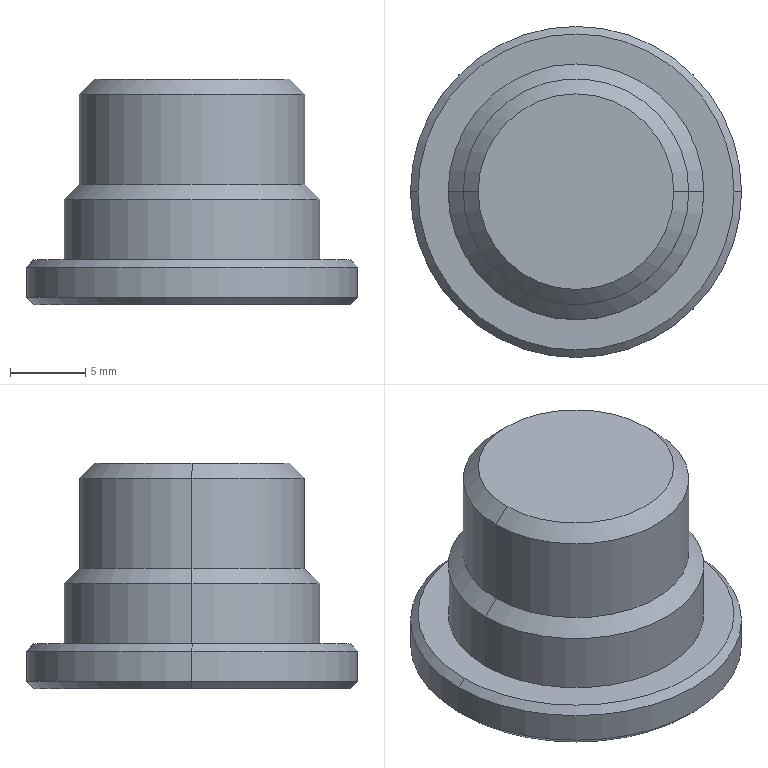Part | SolidWorks | features Chamfer 2, Revolution 1 | 1 solid | 17 faces | box 22 x 22 x 15 mm | volume 3447 mm3 | cone 8 | cylinder 6 | plane 3 | commonest cylinder face diameters 15 x2 17 x2 22 x2
STEP:
#1=CARTESIAN_POINT('',(10.5,0.,-12.));
#2=VERTEX_POINT('',#1);
#3=CARTESIAN_POINT('',(-10.5,0.,-12.));
#4=VERTEX_POINT('',#3);
#5=CARTESIAN_POINT('',(0.,0.,-12.));
#6=DIRECTION('',(0.,0.,1.));
#7=DIRECTION('',(-1.,0.,0.));
#8=AXIS2_PLACEMENT_3D('',#5,#6,#7);
#9=CIRCLE('',#8,10.5);
#10=EDGE_CURVE('',#2,#4,#9,.T.);
#11=ORIENTED_EDGE('',*,*,#10,.F.);
#12=CARTESIAN_POINT('',(11.,0.,-12.5));
#13=VERTEX_POINT('',#12);
#14=CARTESIAN_POINT('',(10.5,0.,-12.));
#15=DIRECTION('',(0.7071,0.,-0.7071));
#16=VECTOR('',#15,1000.);
#17=LINE('',#14,#16);
#18=EDGE_CURVE('',#2,#13,#17,.T.);
#19=ORIENTED_EDGE('',*,*,#18,.T.);
#20=CARTESIAN_POINT('',(-11.,0.,-12.5));
#21=VERTEX_POINT('',#20);
#22=CARTESIAN_POINT('',(0.,0.,-12.5));
#23=DIRECTION('',(0.,0.,-1.));
#24=DIRECTION('',(-1.,0.,0.));
#25=AXIS2_PLACEMENT_3D('',#22,#23,#24);
#26=CIRCLE('',#25,11.);
#27=EDGE_CURVE('',#21,#13,#26,.T.);
#28=ORIENTED_EDGE('',*,*,#27,.F.);
#29=CARTESIAN_POINT('',(-10.5,0.,-12.));
#30=DIRECTION('',(-0.7071,0.,-0.7071));
#31=VECTOR('',#30,1000.);
#32=LINE('',#29,#31);
#33=EDGE_CURVE('',#4,#21,#32,.T.);
#34=ORIENTED_EDGE('',*,*,#33,.F.);
#35=EDGE_LOOP('',(#11,#19,#28,#34));
#36=FACE_OUTER_BOUND('',#35,.T.);
#37=CARTESIAN_POINT('',(0.,0.,-12.));
#38=DIRECTION('',(0.,0.,-1.));
#39=DIRECTION('',(-1.,0.,0.));
#40=AXIS2_PLACEMENT_3D('',#37,#38,#39);
#41=CONICAL_SURFACE('',#40,10.5,0.7854);
#42=ADVANCED_FACE('',(#36),#41,.T.);
#43=CARTESIAN_POINT('',(-10.5,0.,-15.));
#44=VERTEX_POINT('',#43);
#45=CARTESIAN_POINT('',(10.5,0.,-15.));
#46=VERTEX_POINT('',#45);
#47=CARTESIAN_POINT('',(0.,0.,-15.));
#48=DIRECTION('',(0.,0.,-1.));
#49=DIRECTION('',(1.,0.,0.));
#50=AXIS2_PLACEMENT_3D('',#47,#48,#49);
#51=CIRCLE('',#50,10.5);
#52=EDGE_CURVE('',#44,#46,#51,.T.);
#53=ORIENTED_EDGE('',*,*,#52,.F.);
#54=CARTESIAN_POINT('',(-11.,0.,-14.5));
#55=VERTEX_POINT('',#54);
#56=CARTESIAN_POINT('',(-11.,0.,-14.5));
#57=DIRECTION('',(-0.7071,0.,0.7071));
#58=VECTOR('',#57,1000.);
#59=LINE('',#56,#58);
#60=EDGE_CURVE('',#44,#55,#59,.T.);
#61=ORIENTED_EDGE('',*,*,#60,.T.);
#62=CARTESIAN_POINT('',(11.,0.,-14.5));
#63=VERTEX_POINT('',#62);
#64=CARTESIAN_POINT('',(0.,0.,-14.5));
#65=DIRECTION('',(0.,0.,1.));
#66=DIRECTION('',(1.,0.,0.));
#67=AXIS2_PLACEMENT_3D('',#64,#65,#66);
#68=CIRCLE('',#67,11.);
#69=EDGE_CURVE('',#63,#55,#68,.T.);
#70=ORIENTED_EDGE('',*,*,#69,.F.);
#71=CARTESIAN_POINT('',(11.,0.,-14.5));
#72=DIRECTION('',(0.7071,0.,0.7071));
#73=VECTOR('',#72,1000.);
#74=LINE('',#71,#73);
#75=EDGE_CURVE('',#46,#63,#74,.T.);
#76=ORIENTED_EDGE('',*,*,#75,.F.);
#77=EDGE_LOOP('',(#53,#61,#70,#76));
#78=FACE_OUTER_BOUND('',#77,.T.);
#79=CARTESIAN_POINT('',(0.,0.,-14.5));
#80=DIRECTION('',(0.,0.,1.));
#81=DIRECTION('',(1.,0.,0.));
#82=AXIS2_PLACEMENT_3D('',#79,#80,#81);
#83=CONICAL_SURFACE('',#82,11.,0.7854);
#84=ADVANCED_FACE('',(#78),#83,.T.);
#85=CARTESIAN_POINT('',(6.5,0.,0.));
#86=VERTEX_POINT('',#85);
#87=CARTESIAN_POINT('',(-6.5,0.,0.));
#88=VERTEX_POINT('',#87);
#89=CARTESIAN_POINT('',(0.,0.,0.));
#90=DIRECTION('',(0.,0.,1.));
#91=DIRECTION('',(-1.,0.,0.));
#92=AXIS2_PLACEMENT_3D('',#89,#90,#91);
#93=CIRCLE('',#92,6.5);
#94=EDGE_CURVE('',#86,#88,#93,.T.);
#95=ORIENTED_EDGE('',*,*,#94,.F.);
#96=CARTESIAN_POINT('',(7.5,0.,-1.));
#97=VERTEX_POINT('',#96);
#98=CARTESIAN_POINT('',(6.5,0.,0.));
#99=DIRECTION('',(0.7071,0.,-0.7071));
#100=VECTOR('',#99,1000.);
#101=LINE('',#98,#100);
#102=EDGE_CURVE('',#86,#97,#101,.T.);
#103=ORIENTED_EDGE('',*,*,#102,.T.);
#104=CARTESIAN_POINT('',(-7.5,0.,-1.));
#105=VERTEX_POINT('',#104);
#106=CARTESIAN_POINT('',(0.,0.,-1.));
#107=DIRECTION('',(0.,0.,-1.));
#108=DIRECTION('',(-1.,0.,0.));
#109=AXIS2_PLACEMENT_3D('',#106,#107,#108);
#110=CIRCLE('',#109,7.5);
#111=EDGE_CURVE('',#105,#97,#110,.T.);
#112=ORIENTED_EDGE('',*,*,#111,.F.);
#113=CARTESIAN_POINT('',(-6.5,0.,0.));
#114=DIRECTION('',(-0.7071,0.,-0.7071));
#115=VECTOR('',#114,1000.);
#116=LINE('',#113,#115);
#117=EDGE_CURVE('',#88,#105,#116,.T.);
#118=ORIENTED_EDGE('',*,*,#117,.F.);
#119=EDGE_LOOP('',(#95,#103,#112,#118));
#120=FACE_OUTER_BOUND('',#119,.T.);
#121=CARTESIAN_POINT('',(0.,0.,0.));
#122=DIRECTION('',(0.,0.,-1.));
#123=DIRECTION('',(-1.,0.,0.));
#124=AXIS2_PLACEMENT_3D('',#121,#122,#123);
#125=CONICAL_SURFACE('',#124,6.5,0.7854);
#126=ADVANCED_FACE('',(#120),#125,.T.);
#127=CARTESIAN_POINT('',(7.5,0.,-7.));
#128=VERTEX_POINT('',#127);
#129=CARTESIAN_POINT('',(-7.5,0.,-7.));
#130=VERTEX_POINT('',#129);
#131=CARTESIAN_POINT('',(0.,0.,-7.));
#132=DIRECTION('',(0.,0.,1.));
#133=DIRECTION('',(1.,0.,0.));
#134=AXIS2_PLACEMENT_3D('',#131,#132,#133);
#135=CIRCLE('',#134,7.5);
#136=EDGE_CURVE('',#128,#130,#135,.T.);
#137=ORIENTED_EDGE('',*,*,#136,.F.);
#138=CARTESIAN_POINT('',(8.5,0.,-8.));
#139=VERTEX_POINT('',#138);
#140=CARTESIAN_POINT('',(7.5,0.,-7.));
#141=DIRECTION('',(0.7071,0.,-0.7071));
#142=VECTOR('',#141,1000.);
#143=LINE('',#140,#142);
#144=EDGE_CURVE('',#128,#139,#143,.T.);
#145=ORIENTED_EDGE('',*,*,#144,.T.);
#146=CARTESIAN_POINT('',(-8.5,0.,-8.));
#147=VERTEX_POINT('',#146);
#148=CARTESIAN_POINT('',(0.,0.,-8.));
#149=DIRECTION('',(0.,0.,-1.));
#150=DIRECTION('',(-1.,0.,0.));
#151=AXIS2_PLACEMENT_3D('',#148,#149,#150);
#152=CIRCLE('',#151,8.5);
#153=EDGE_CURVE('',#147,#139,#152,.T.);
#154=ORIENTED_EDGE('',*,*,#153,.F.);
#155=CARTESIAN_POINT('',(-7.5,0.,-7.));
#156=DIRECTION('',(-0.7071,0.,-0.7071));
#157=VECTOR('',#156,1000.);
#158=LINE('',#155,#157);
#159=EDGE_CURVE('',#130,#147,#158,.T.);
#160=ORIENTED_EDGE('',*,*,#159,.F.);
#161=EDGE_LOOP('',(#137,#145,#154,#160));
#162=FACE_OUTER_BOUND('',#161,.T.);
#163=CARTESIAN_POINT('',(0.,0.,-7.));
#164=DIRECTION('',(0.,0.,-1.));
#165=DIRECTION('',(-1.,0.,0.));
#166=AXIS2_PLACEMENT_3D('',#163,#164,#165);
#167=CONICAL_SURFACE('',#166,7.5,0.7854);
#168=ADVANCED_FACE('',(#162),#167,.T.);
#169=ORIENTED_EDGE('',*,*,#69,.T.);
#170=CARTESIAN_POINT('',(-11.,0.,0.));
#171=DIRECTION('',(0.,0.,1.));
#172=VECTOR('',#171,1000.);
#173=LINE('',#170,#172);
#174=EDGE_CURVE('',#55,#21,#173,.T.);
#175=ORIENTED_EDGE('',*,*,#174,.T.);
#176=ORIENTED_EDGE('',*,*,#27,.T.);
#177=CARTESIAN_POINT('',(11.,0.,0.));
#178=DIRECTION('',(0.,0.,1.));
#179=VECTOR('',#178,1000.);
#180=LINE('',#177,#179);
#181=EDGE_CURVE('',#63,#13,#180,.T.);
#182=ORIENTED_EDGE('',*,*,#181,.F.);
#183=EDGE_LOOP('',(#169,#175,#176,#182));
#184=FACE_OUTER_BOUND('',#183,.T.);
#185=CARTESIAN_POINT('',(0.,0.,0.));
#186=DIRECTION('',(0.,0.,1.));
#187=DIRECTION('',(1.,0.,0.));
#188=AXIS2_PLACEMENT_3D('',#185,#186,#187);
#189=CYLINDRICAL_SURFACE('',#188,11.);
#190=ADVANCED_FACE('',(#184),#189,.T.);
#191=CARTESIAN_POINT('',(8.5,0.,-12.));
#192=VERTEX_POINT('',#191);
#193=CARTESIAN_POINT('',(-8.5,0.,-12.));
#194=VERTEX_POINT('',#193);
#195=CARTESIAN_POINT('',(0.,0.,-12.));
#196=DIRECTION('',(0.,0.,1.));
#197=DIRECTION('',(1.,0.,0.));
#198=AXIS2_PLACEMENT_3D('',#195,#196,#197);
#199=CIRCLE('',#198,8.5);
#200=EDGE_CURVE('',#192,#194,#199,.T.);
#201=ORIENTED_EDGE('',*,*,#200,.T.);
#202=CARTESIAN_POINT('',(-8.5,0.,0.));
#203=DIRECTION('',(0.,0.,1.));
#204=VECTOR('',#203,1000.);
#205=LINE('',#202,#204);
#206=EDGE_CURVE('',#194,#147,#205,.T.);
#207=ORIENTED_EDGE('',*,*,#206,.T.);
#208=ORIENTED_EDGE('',*,*,#153,.T.);
#209=CARTESIAN_POINT('',(8.5,0.,0.));
#210=DIRECTION('',(0.,0.,1.));
#211=VECTOR('',#210,1000.);
#212=LINE('',#209,#211);
#213=EDGE_CURVE('',#192,#139,#212,.T.);
#214=ORIENTED_EDGE('',*,*,#213,.F.);
#215=EDGE_LOOP('',(#201,#207,#208,#214));
#216=FACE_OUTER_BOUND('',#215,.T.);
#217=CARTESIAN_POINT('',(0.,0.,0.));
#218=DIRECTION('',(0.,0.,1.));
#219=DIRECTION('',(1.,0.,0.));
#220=AXIS2_PLACEMENT_3D('',#217,#218,#219);
#221=CYLINDRICAL_SURFACE('',#220,8.5);
#222=ADVANCED_FACE('',(#216),#221,.T.);
#223=ORIENTED_EDGE('',*,*,#136,.T.);
#224=CARTESIAN_POINT('',(-7.5,0.,0.));
#225=DIRECTION('',(0.,0.,1.));
#226=VECTOR('',#225,1000.);
#227=LINE('',#224,#226);
#228=EDGE_CURVE('',#130,#105,#227,.T.);
#229=ORIENTED_EDGE('',*,*,#228,.T.);
#230=ORIENTED_EDGE('',*,*,#111,.T.);
#231=CARTESIAN_POINT('',(7.5,0.,0.));
#232=DIRECTION('',(0.,0.,1.));
#233=VECTOR('',#232,1000.);
#234=LINE('',#231,#233);
#235=EDGE_CURVE('',#128,#97,#234,.T.);
#236=ORIENTED_EDGE('',*,*,#235,.F.);
#237=EDGE_LOOP('',(#223,#229,#230,#236));
#238=FACE_OUTER_BOUND('',#237,.T.);
#239=CARTESIAN_POINT('',(0.,0.,0.));
#240=DIRECTION('',(0.,0.,1.));
#241=DIRECTION('',(1.,0.,0.));
#242=AXIS2_PLACEMENT_3D('',#239,#240,#241);
#243=CYLINDRICAL_SURFACE('',#242,7.5);
#244=ADVANCED_FACE('',(#238),#243,.T.);
#245=CARTESIAN_POINT('',(0.,0.,0.));
#246=DIRECTION('',(0.,0.,1.));
#247=DIRECTION('',(-1.,0.,0.));
#248=AXIS2_PLACEMENT_3D('',#245,#246,#247);
#249=CIRCLE('',#248,6.5);
#250=EDGE_CURVE('',#88,#86,#249,.T.);
#251=ORIENTED_EDGE('',*,*,#250,.T.);
#252=ORIENTED_EDGE('',*,*,#94,.T.);
#253=EDGE_LOOP('',(#251,#252));
#254=FACE_OUTER_BOUND('',#253,.T.);
#255=CARTESIAN_POINT('',(0.,0.,0.));
#256=DIRECTION('',(0.,0.,-1.));
#257=DIRECTION('',(-1.,0.,0.));
#258=AXIS2_PLACEMENT_3D('',#255,#256,#257);
#259=PLANE('',#258);
#260=ADVANCED_FACE('',(#254),#259,.F.);
#261=ORIENTED_EDGE('',*,*,#228,.F.);
#262=CARTESIAN_POINT('',(0.,0.,-7.));
#263=DIRECTION('',(0.,0.,1.));
#264=DIRECTION('',(1.,0.,0.));
#265=AXIS2_PLACEMENT_3D('',#262,#263,#264);
#266=CIRCLE('',#265,7.5);
#267=EDGE_CURVE('',#130,#128,#266,.T.);
#268=ORIENTED_EDGE('',*,*,#267,.T.);
#269=ORIENTED_EDGE('',*,*,#235,.T.);
#270=CARTESIAN_POINT('',(0.,0.,-1.));
#271=DIRECTION('',(0.,0.,-1.));
#272=DIRECTION('',(-1.,0.,0.));
#273=AXIS2_PLACEMENT_3D('',#270,#271,#272);
#274=CIRCLE('',#273,7.5);
#275=EDGE_CURVE('',#97,#105,#274,.T.);
#276=ORIENTED_EDGE('',*,*,#275,.T.);
#277=EDGE_LOOP('',(#261,#268,#269,#276));
#278=FACE_OUTER_BOUND('',#277,.T.);
#279=CARTESIAN_POINT('',(0.,0.,0.));
#280=DIRECTION('',(0.,0.,1.));
#281=DIRECTION('',(1.,0.,0.));
#282=AXIS2_PLACEMENT_3D('',#279,#280,#281);
#283=CYLINDRICAL_SURFACE('',#282,7.5);
#284=ADVANCED_FACE('',(#278),#283,.T.);
#285=ORIENTED_EDGE('',*,*,#206,.F.);
#286=CARTESIAN_POINT('',(0.,0.,-12.));
#287=DIRECTION('',(0.,0.,1.));
#288=DIRECTION('',(1.,0.,0.));
#289=AXIS2_PLACEMENT_3D('',#286,#287,#288);
#290=CIRCLE('',#289,8.5);
#291=EDGE_CURVE('',#194,#192,#290,.T.);
#292=ORIENTED_EDGE('',*,*,#291,.T.);
#293=ORIENTED_EDGE('',*,*,#213,.T.);
#294=CARTESIAN_POINT('',(0.,0.,-8.));
#295=DIRECTION('',(0.,0.,-1.));
#296=DIRECTION('',(-1.,0.,0.));
#297=AXIS2_PLACEMENT_3D('',#294,#295,#296);
#298=CIRCLE('',#297,8.5);
#299=EDGE_CURVE('',#139,#147,#298,.T.);
#300=ORIENTED_EDGE('',*,*,#299,.T.);
#301=EDGE_LOOP('',(#285,#292,#293,#300));
#302=FACE_OUTER_BOUND('',#301,.T.);
#303=CARTESIAN_POINT('',(0.,0.,0.));
#304=DIRECTION('',(0.,0.,1.));
#305=DIRECTION('',(1.,0.,0.));
#306=AXIS2_PLACEMENT_3D('',#303,#304,#305);
#307=CYLINDRICAL_SURFACE('',#306,8.5);
#308=ADVANCED_FACE('',(#302),#307,.T.);
#309=CARTESIAN_POINT('',(0.,0.,-12.));
#310=DIRECTION('',(0.,0.,1.));
#311=DIRECTION('',(-1.,0.,0.));
#312=AXIS2_PLACEMENT_3D('',#309,#310,#311);
#313=CIRCLE('',#312,10.5);
#314=EDGE_CURVE('',#4,#2,#313,.T.);
#315=ORIENTED_EDGE('',*,*,#314,.T.);
#316=ORIENTED_EDGE('',*,*,#10,.T.);
#317=EDGE_LOOP('',(#315,#316));
#318=FACE_OUTER_BOUND('',#317,.T.);
#319=ORIENTED_EDGE('',*,*,#200,.F.);
#320=ORIENTED_EDGE('',*,*,#291,.F.);
#321=EDGE_LOOP('',(#319,#320));
#322=FACE_BOUND('',#321,.T.);
#323=CARTESIAN_POINT('',(0.,8.5,-12.));
#324=DIRECTION('',(0.,0.,-1.));
#325=DIRECTION('',(-1.,0.,0.));
#326=AXIS2_PLACEMENT_3D('',#323,#324,#325);
#327=PLANE('',#326);
#328=ADVANCED_FACE('',(#318,#322),#327,.F.);
#329=ORIENTED_EDGE('',*,*,#174,.F.);
#330=CARTESIAN_POINT('',(0.,0.,-14.5));
#331=DIRECTION('',(0.,0.,1.));
#332=DIRECTION('',(1.,0.,0.));
#333=AXIS2_PLACEMENT_3D('',#330,#331,#332);
#334=CIRCLE('',#333,11.);
#335=EDGE_CURVE('',#55,#63,#334,.T.);
#336=ORIENTED_EDGE('',*,*,#335,.T.);
#337=ORIENTED_EDGE('',*,*,#181,.T.);
#338=CARTESIAN_POINT('',(0.,0.,-12.5));
#339=DIRECTION('',(0.,0.,-1.));
#340=DIRECTION('',(-1.,0.,0.));
#341=AXIS2_PLACEMENT_3D('',#338,#339,#340);
#342=CIRCLE('',#341,11.);
#343=EDGE_CURVE('',#13,#21,#342,.T.);
#344=ORIENTED_EDGE('',*,*,#343,.T.);
#345=EDGE_LOOP('',(#329,#336,#337,#344));
#346=FACE_OUTER_BOUND('',#345,.T.);
#347=CARTESIAN_POINT('',(0.,0.,0.));
#348=DIRECTION('',(0.,0.,1.));
#349=DIRECTION('',(1.,0.,0.));
#350=AXIS2_PLACEMENT_3D('',#347,#348,#349);
#351=CYLINDRICAL_SURFACE('',#350,11.);
#352=ADVANCED_FACE('',(#346),#351,.T.);
#353=CARTESIAN_POINT('',(0.,0.,-15.));
#354=DIRECTION('',(0.,0.,-1.));
#355=DIRECTION('',(1.,0.,0.));
#356=AXIS2_PLACEMENT_3D('',#353,#354,#355);
#357=CIRCLE('',#356,10.5);
#358=EDGE_CURVE('',#46,#44,#357,.T.);
#359=ORIENTED_EDGE('',*,*,#358,.T.);
#360=ORIENTED_EDGE('',*,*,#52,.T.);
#361=EDGE_LOOP('',(#359,#360));
#362=FACE_OUTER_BOUND('',#361,.T.);
#363=CARTESIAN_POINT('',(0.,11.,-15.));
#364=DIRECTION('',(0.,0.,1.));
#365=DIRECTION('',(1.,0.,0.));
#366=AXIS2_PLACEMENT_3D('',#363,#364,#365);
#367=PLANE('',#366);
#368=ADVANCED_FACE('',(#362),#367,.F.);
#369=ORIENTED_EDGE('',*,*,#144,.F.);
#370=ORIENTED_EDGE('',*,*,#267,.F.);
#371=ORIENTED_EDGE('',*,*,#159,.T.);
#372=ORIENTED_EDGE('',*,*,#299,.F.);
#373=EDGE_LOOP('',(#369,#370,#371,#372));
#374=FACE_OUTER_BOUND('',#373,.T.);
#375=CARTESIAN_POINT('',(0.,0.,-7.));
#376=DIRECTION('',(0.,0.,-1.));
#377=DIRECTION('',(-1.,0.,0.));
#378=AXIS2_PLACEMENT_3D('',#375,#376,#377);
#379=CONICAL_SURFACE('',#378,7.5,0.7854);
#380=ADVANCED_FACE('',(#374),#379,.T.);
#381=ORIENTED_EDGE('',*,*,#102,.F.);
#382=ORIENTED_EDGE('',*,*,#250,.F.);
#383=ORIENTED_EDGE('',*,*,#117,.T.);
#384=ORIENTED_EDGE('',*,*,#275,.F.);
#385=EDGE_LOOP('',(#381,#382,#383,#384));
#386=FACE_OUTER_BOUND('',#385,.T.);
#387=CARTESIAN_POINT('',(0.,0.,0.));
#388=DIRECTION('',(0.,0.,-1.));
#389=DIRECTION('',(-1.,0.,0.));
#390=AXIS2_PLACEMENT_3D('',#387,#388,#389);
#391=CONICAL_SURFACE('',#390,6.5,0.7854);
#392=ADVANCED_FACE('',(#386),#391,.T.);
#393=ORIENTED_EDGE('',*,*,#60,.F.);
#394=ORIENTED_EDGE('',*,*,#358,.F.);
#395=ORIENTED_EDGE('',*,*,#75,.T.);
#396=ORIENTED_EDGE('',*,*,#335,.F.);
#397=EDGE_LOOP('',(#393,#394,#395,#396));
#398=FACE_OUTER_BOUND('',#397,.T.);
#399=CARTESIAN_POINT('',(0.,0.,-14.5));
#400=DIRECTION('',(0.,0.,1.));
#401=DIRECTION('',(1.,0.,0.));
#402=AXIS2_PLACEMENT_3D('',#399,#400,#401);
#403=CONICAL_SURFACE('',#402,11.,0.7854);
#404=ADVANCED_FACE('',(#398),#403,.T.);
#405=ORIENTED_EDGE('',*,*,#18,.F.);
#406=ORIENTED_EDGE('',*,*,#314,.F.);
#407=ORIENTED_EDGE('',*,*,#33,.T.);
#408=ORIENTED_EDGE('',*,*,#343,.F.);
#409=EDGE_LOOP('',(#405,#406,#407,#408));
#410=FACE_OUTER_BOUND('',#409,.T.);
#411=CARTESIAN_POINT('',(0.,0.,-12.));
#412=DIRECTION('',(0.,0.,-1.));
#413=DIRECTION('',(-1.,0.,0.));
#414=AXIS2_PLACEMENT_3D('',#411,#412,#413);
#415=CONICAL_SURFACE('',#414,10.5,0.7854);
#416=ADVANCED_FACE('',(#410),#415,.T.);
#417=CLOSED_SHELL('',(#42,#84,#126,#168,#190,#222,#244,#260,#284,#308,#328,#352,#368,#380,#392,#404,#416));
#418=MANIFOLD_SOLID_BREP('',#417);
#419=CARTESIAN_POINT('',(0.,0.,0.));
#420=DIRECTION('',(0.,0.,1.));
#421=DIRECTION('',(1.,0.,0.));
#422=AXIS2_PLACEMENT_3D('',#419,#420,#421);
#423=(LENGTH_UNIT()NAMED_UNIT(*)SI_UNIT(.MILLI.,.METRE.));
#424=UNCERTAINTY_MEASURE_WITH_UNIT(LENGTH_MEASURE(0.00001),#423,'','');
#425=(NAMED_UNIT(*)PLANE_ANGLE_UNIT()SI_UNIT($,.RADIAN.));
#426=(NAMED_UNIT(*)SI_UNIT($,.STERADIAN.)SOLID_ANGLE_UNIT());
#427=(GEOMETRIC_REPRESENTATION_CONTEXT(3)GLOBAL_UNCERTAINTY_ASSIGNED_CONTEXT((#424))GLOBAL_UNIT_ASSIGNED_CONTEXT((#423,#425,#426))REPRESENTATION_CONTEXT('',''));
#428=ADVANCED_BREP_SHAPE_REPRESENTATION('',(#418,#422),#427);